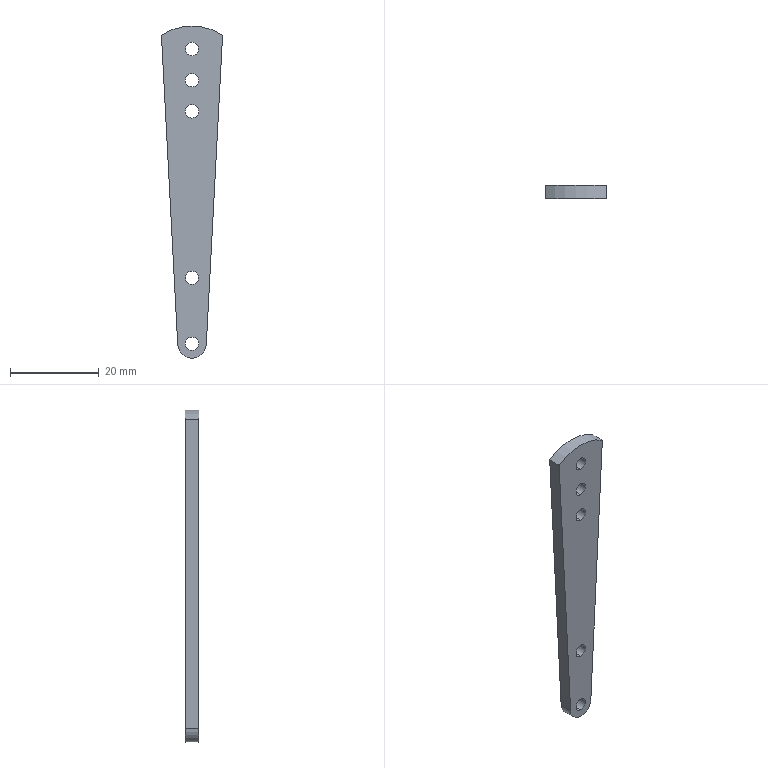Part | SolidWorks | features ICE 3, BaseBody 1 | 1 solid | 16 faces | box 13.735 x 3 x 74.656 mm | volume 2101 mm3 | cylinder 12 | plane 4 | commonest cylinder face diameters 3 x10 6.445 x1 24.375 x1
STEP:
#1=CARTESIAN_POINT('',(40.836,0.,-86.129));
#2=VERTEX_POINT('',#1);
#3=CARTESIAN_POINT('',(40.836,0.,-89.129));
#4=VERTEX_POINT('',#3);
#5=CARTESIAN_POINT('',(40.836,0.,-87.629));
#6=DIRECTION('',(0.,-1.,0.));
#7=DIRECTION('',(0.,0.,1.));
#8=AXIS2_PLACEMENT_3D('',#5,#6,#7);
#9=CIRCLE('',#8,1.5);
#10=EDGE_CURVE('',#2,#4,#9,.T.);
#11=ORIENTED_EDGE('',*,*,#10,.T.);
#12=CARTESIAN_POINT('',(40.836,3.,-89.129));
#13=VERTEX_POINT('',#12);
#14=CARTESIAN_POINT('',(40.836,-19.541,-89.129));
#15=DIRECTION('',(0.,1.,0.));
#16=VECTOR('',#15,1000.);
#17=LINE('',#14,#16);
#18=EDGE_CURVE('',#4,#13,#17,.T.);
#19=ORIENTED_EDGE('',*,*,#18,.T.);
#20=CARTESIAN_POINT('',(40.836,3.,-86.129));
#21=VERTEX_POINT('',#20);
#22=CARTESIAN_POINT('',(40.836,3.,-87.629));
#23=DIRECTION('',(0.,1.,0.));
#24=DIRECTION('',(0.,0.,1.));
#25=AXIS2_PLACEMENT_3D('',#22,#23,#24);
#26=CIRCLE('',#25,1.5);
#27=EDGE_CURVE('',#13,#21,#26,.T.);
#28=ORIENTED_EDGE('',*,*,#27,.T.);
#29=CARTESIAN_POINT('',(40.836,-19.541,-86.129));
#30=DIRECTION('',(0.,1.,0.));
#31=VECTOR('',#30,1000.);
#32=LINE('',#29,#31);
#33=EDGE_CURVE('',#2,#21,#32,.T.);
#34=ORIENTED_EDGE('',*,*,#33,.F.);
#35=EDGE_LOOP('',(#11,#19,#28,#34));
#36=FACE_OUTER_BOUND('',#35,.T.);
#37=CARTESIAN_POINT('',(40.836,-19.541,-87.629));
#38=DIRECTION('',(0.,1.,0.));
#39=DIRECTION('',(0.,0.,1.));
#40=AXIS2_PLACEMENT_3D('',#37,#38,#39);
#41=CYLINDRICAL_SURFACE('',#40,1.5);
#42=ADVANCED_FACE('',(#36),#41,.F.);
#43=CARTESIAN_POINT('',(40.836,0.,-71.309));
#44=VERTEX_POINT('',#43);
#45=CARTESIAN_POINT('',(40.836,0.,-74.309));
#46=VERTEX_POINT('',#45);
#47=CARTESIAN_POINT('',(40.836,0.,-72.809));
#48=DIRECTION('',(0.,-1.,0.));
#49=DIRECTION('',(0.,0.,1.));
#50=AXIS2_PLACEMENT_3D('',#47,#48,#49);
#51=CIRCLE('',#50,1.5);
#52=EDGE_CURVE('',#44,#46,#51,.T.);
#53=ORIENTED_EDGE('',*,*,#52,.T.);
#54=CARTESIAN_POINT('',(40.836,3.,-74.309));
#55=VERTEX_POINT('',#54);
#56=CARTESIAN_POINT('',(40.836,-39.423,-74.309));
#57=DIRECTION('',(0.,1.,0.));
#58=VECTOR('',#57,1000.);
#59=LINE('',#56,#58);
#60=EDGE_CURVE('',#46,#55,#59,.T.);
#61=ORIENTED_EDGE('',*,*,#60,.T.);
#62=CARTESIAN_POINT('',(40.836,3.,-71.309));
#63=VERTEX_POINT('',#62);
#64=CARTESIAN_POINT('',(40.836,3.,-72.809));
#65=DIRECTION('',(0.,1.,0.));
#66=DIRECTION('',(0.,0.,1.));
#67=AXIS2_PLACEMENT_3D('',#64,#65,#66);
#68=CIRCLE('',#67,1.5);
#69=EDGE_CURVE('',#55,#63,#68,.T.);
#70=ORIENTED_EDGE('',*,*,#69,.T.);
#71=CARTESIAN_POINT('',(40.836,-39.423,-71.309));
#72=DIRECTION('',(0.,1.,0.));
#73=VECTOR('',#72,1000.);
#74=LINE('',#71,#73);
#75=EDGE_CURVE('',#44,#63,#74,.T.);
#76=ORIENTED_EDGE('',*,*,#75,.F.);
#77=EDGE_LOOP('',(#53,#61,#70,#76));
#78=FACE_OUTER_BOUND('',#77,.T.);
#79=CARTESIAN_POINT('',(40.836,-39.423,-72.809));
#80=DIRECTION('',(0.,1.,0.));
#81=DIRECTION('',(0.,0.,1.));
#82=AXIS2_PLACEMENT_3D('',#79,#80,#81);
#83=CYLINDRICAL_SURFACE('',#82,1.5);
#84=ADVANCED_FACE('',(#78),#83,.F.);
#85=CARTESIAN_POINT('',(40.836,3.,-26.883));
#86=VERTEX_POINT('',#85);
#87=CARTESIAN_POINT('',(40.836,3.,-29.883));
#88=VERTEX_POINT('',#87);
#89=CARTESIAN_POINT('',(40.836,3.,-28.383));
#90=DIRECTION('',(0.,-1.,0.));
#91=DIRECTION('',(0.,0.,-1.));
#92=AXIS2_PLACEMENT_3D('',#89,#90,#91);
#93=CIRCLE('',#92,1.5);
#94=EDGE_CURVE('',#86,#88,#93,.T.);
#95=ORIENTED_EDGE('',*,*,#94,.F.);
#96=CARTESIAN_POINT('',(40.836,0.,-26.883));
#97=VERTEX_POINT('',#96);
#98=CARTESIAN_POINT('',(40.836,3.,-26.883));
#99=DIRECTION('',(0.,-1.,0.));
#100=VECTOR('',#99,1000.);
#101=LINE('',#98,#100);
#102=EDGE_CURVE('',#86,#97,#101,.T.);
#103=ORIENTED_EDGE('',*,*,#102,.T.);
#104=CARTESIAN_POINT('',(40.836,0.,-29.883));
#105=VERTEX_POINT('',#104);
#106=CARTESIAN_POINT('',(40.836,0.,-28.383));
#107=DIRECTION('',(0.,-1.,0.));
#108=DIRECTION('',(0.,0.,-1.));
#109=AXIS2_PLACEMENT_3D('',#106,#107,#108);
#110=CIRCLE('',#109,1.5);
#111=EDGE_CURVE('',#97,#105,#110,.T.);
#112=ORIENTED_EDGE('',*,*,#111,.T.);
#113=CARTESIAN_POINT('',(40.836,3.,-29.883));
#114=DIRECTION('',(0.,-1.,0.));
#115=VECTOR('',#114,1000.);
#116=LINE('',#113,#115);
#117=EDGE_CURVE('',#88,#105,#116,.T.);
#118=ORIENTED_EDGE('',*,*,#117,.F.);
#119=EDGE_LOOP('',(#95,#103,#112,#118));
#120=FACE_OUTER_BOUND('',#119,.T.);
#121=CARTESIAN_POINT('',(40.836,3.,-28.383));
#122=DIRECTION('',(0.,-1.,0.));
#123=DIRECTION('',(0.,0.,-1.));
#124=AXIS2_PLACEMENT_3D('',#121,#122,#123);
#125=CYLINDRICAL_SURFACE('',#124,1.5);
#126=ADVANCED_FACE('',(#120),#125,.F.);
#127=CARTESIAN_POINT('',(40.836,3.,-19.883));
#128=VERTEX_POINT('',#127);
#129=CARTESIAN_POINT('',(40.836,3.,-22.883));
#130=VERTEX_POINT('',#129);
#131=CARTESIAN_POINT('',(40.836,3.,-21.383));
#132=DIRECTION('',(0.,-1.,0.));
#133=DIRECTION('',(0.,0.,-1.));
#134=AXIS2_PLACEMENT_3D('',#131,#132,#133);
#135=CIRCLE('',#134,1.5);
#136=EDGE_CURVE('',#128,#130,#135,.T.);
#137=ORIENTED_EDGE('',*,*,#136,.F.);
#138=CARTESIAN_POINT('',(40.836,0.,-19.883));
#139=VERTEX_POINT('',#138);
#140=CARTESIAN_POINT('',(40.836,3.,-19.883));
#141=DIRECTION('',(0.,-1.,0.));
#142=VECTOR('',#141,1000.);
#143=LINE('',#140,#142);
#144=EDGE_CURVE('',#128,#139,#143,.T.);
#145=ORIENTED_EDGE('',*,*,#144,.T.);
#146=CARTESIAN_POINT('',(40.836,0.,-22.883));
#147=VERTEX_POINT('',#146);
#148=CARTESIAN_POINT('',(40.836,0.,-21.383));
#149=DIRECTION('',(0.,-1.,0.));
#150=DIRECTION('',(0.,0.,-1.));
#151=AXIS2_PLACEMENT_3D('',#148,#149,#150);
#152=CIRCLE('',#151,1.5);
#153=EDGE_CURVE('',#139,#147,#152,.T.);
#154=ORIENTED_EDGE('',*,*,#153,.T.);
#155=CARTESIAN_POINT('',(40.836,3.,-22.883));
#156=DIRECTION('',(0.,-1.,0.));
#157=VECTOR('',#156,1000.);
#158=LINE('',#155,#157);
#159=EDGE_CURVE('',#130,#147,#158,.T.);
#160=ORIENTED_EDGE('',*,*,#159,.F.);
#161=EDGE_LOOP('',(#137,#145,#154,#160));
#162=FACE_OUTER_BOUND('',#161,.T.);
#163=CARTESIAN_POINT('',(40.836,3.,-21.383));
#164=DIRECTION('',(0.,-1.,0.));
#165=DIRECTION('',(0.,0.,-1.));
#166=AXIS2_PLACEMENT_3D('',#163,#164,#165);
#167=CYLINDRICAL_SURFACE('',#166,1.5);
#168=ADVANCED_FACE('',(#162),#167,.F.);
#169=CARTESIAN_POINT('',(40.836,3.,-33.883));
#170=VERTEX_POINT('',#169);
#171=CARTESIAN_POINT('',(40.836,3.,-36.883));
#172=VERTEX_POINT('',#171);
#173=CARTESIAN_POINT('',(40.836,3.,-35.383));
#174=DIRECTION('',(0.,-1.,0.));
#175=DIRECTION('',(0.,0.,-1.));
#176=AXIS2_PLACEMENT_3D('',#173,#174,#175);
#177=CIRCLE('',#176,1.5);
#178=EDGE_CURVE('',#170,#172,#177,.T.);
#179=ORIENTED_EDGE('',*,*,#178,.F.);
#180=CARTESIAN_POINT('',(40.836,0.,-33.883));
#181=VERTEX_POINT('',#180);
#182=CARTESIAN_POINT('',(40.836,3.,-33.883));
#183=DIRECTION('',(0.,-1.,0.));
#184=VECTOR('',#183,1000.);
#185=LINE('',#182,#184);
#186=EDGE_CURVE('',#170,#181,#185,.T.);
#187=ORIENTED_EDGE('',*,*,#186,.T.);
#188=CARTESIAN_POINT('',(40.836,0.,-36.883));
#189=VERTEX_POINT('',#188);
#190=CARTESIAN_POINT('',(40.836,0.,-35.383));
#191=DIRECTION('',(0.,-1.,0.));
#192=DIRECTION('',(0.,0.,-1.));
#193=AXIS2_PLACEMENT_3D('',#190,#191,#192);
#194=CIRCLE('',#193,1.5);
#195=EDGE_CURVE('',#181,#189,#194,.T.);
#196=ORIENTED_EDGE('',*,*,#195,.T.);
#197=CARTESIAN_POINT('',(40.836,3.,-36.883));
#198=DIRECTION('',(0.,-1.,0.));
#199=VECTOR('',#198,1000.);
#200=LINE('',#197,#199);
#201=EDGE_CURVE('',#172,#189,#200,.T.);
#202=ORIENTED_EDGE('',*,*,#201,.F.);
#203=EDGE_LOOP('',(#179,#187,#196,#202));
#204=FACE_OUTER_BOUND('',#203,.T.);
#205=CARTESIAN_POINT('',(40.836,3.,-35.383));
#206=DIRECTION('',(0.,-1.,0.));
#207=DIRECTION('',(0.,0.,-1.));
#208=AXIS2_PLACEMENT_3D('',#205,#206,#207);
#209=CYLINDRICAL_SURFACE('',#208,1.5);
#210=ADVANCED_FACE('',(#204),#209,.F.);
#211=CARTESIAN_POINT('',(44.054,3.,-87.798));
#212=VERTEX_POINT('',#211);
#213=CARTESIAN_POINT('',(47.703,3.,-18.315));
#214=VERTEX_POINT('',#213);
#215=CARTESIAN_POINT('',(45.586,3.,-58.633));
#216=DIRECTION('',(0.05245,0.,0.9986));
#217=VECTOR('',#216,1000.);
#218=LINE('',#215,#217);
#219=EDGE_CURVE('',#212,#214,#218,.T.);
#220=ORIENTED_EDGE('',*,*,#219,.F.);
#221=CARTESIAN_POINT('',(37.617,3.,-87.798));
#222=VERTEX_POINT('',#221);
#223=CARTESIAN_POINT('',(40.836,3.,-87.629));
#224=DIRECTION('',(0.,1.,0.));
#225=DIRECTION('',(0.,0.,-1.));
#226=AXIS2_PLACEMENT_3D('',#223,#224,#225);
#227=CIRCLE('',#226,3.223);
#228=EDGE_CURVE('',#212,#222,#227,.T.);
#229=ORIENTED_EDGE('',*,*,#228,.T.);
#230=CARTESIAN_POINT('',(33.968,3.,-18.315));
#231=VERTEX_POINT('',#230);
#232=CARTESIAN_POINT('',(36.086,3.,-58.633));
#233=DIRECTION('',(0.05245,0.,-0.9986));
#234=VECTOR('',#233,1000.);
#235=LINE('',#232,#234);
#236=EDGE_CURVE('',#231,#222,#235,.T.);
#237=ORIENTED_EDGE('',*,*,#236,.F.);
#238=CARTESIAN_POINT('',(40.836,3.,-28.383));
#239=DIRECTION('',(0.,-1.,0.));
#240=DIRECTION('',(0.,0.,-1.));
#241=AXIS2_PLACEMENT_3D('',#238,#239,#240);
#242=CIRCLE('',#241,12.188);
#243=EDGE_CURVE('',#214,#231,#242,.T.);
#244=ORIENTED_EDGE('',*,*,#243,.F.);
#245=EDGE_LOOP('',(#220,#229,#237,#244));
#246=FACE_OUTER_BOUND('',#245,.T.);
#247=CARTESIAN_POINT('',(40.836,3.,-35.383));
#248=DIRECTION('',(0.,-1.,0.));
#249=DIRECTION('',(0.,0.,-1.));
#250=AXIS2_PLACEMENT_3D('',#247,#248,#249);
#251=CIRCLE('',#250,1.5);
#252=EDGE_CURVE('',#172,#170,#251,.T.);
#253=ORIENTED_EDGE('',*,*,#252,.T.);
#254=ORIENTED_EDGE('',*,*,#178,.T.);
#255=EDGE_LOOP('',(#253,#254));
#256=FACE_BOUND('',#255,.T.);
#257=CARTESIAN_POINT('',(40.836,3.,-21.383));
#258=DIRECTION('',(0.,-1.,0.));
#259=DIRECTION('',(0.,0.,-1.));
#260=AXIS2_PLACEMENT_3D('',#257,#258,#259);
#261=CIRCLE('',#260,1.5);
#262=EDGE_CURVE('',#130,#128,#261,.T.);
#263=ORIENTED_EDGE('',*,*,#262,.T.);
#264=ORIENTED_EDGE('',*,*,#136,.T.);
#265=EDGE_LOOP('',(#263,#264));
#266=FACE_BOUND('',#265,.T.);
#267=CARTESIAN_POINT('',(40.836,3.,-28.383));
#268=DIRECTION('',(0.,-1.,0.));
#269=DIRECTION('',(0.,0.,-1.));
#270=AXIS2_PLACEMENT_3D('',#267,#268,#269);
#271=CIRCLE('',#270,1.5);
#272=EDGE_CURVE('',#88,#86,#271,.T.);
#273=ORIENTED_EDGE('',*,*,#272,.T.);
#274=ORIENTED_EDGE('',*,*,#94,.T.);
#275=EDGE_LOOP('',(#273,#274));
#276=FACE_BOUND('',#275,.T.);
#277=CARTESIAN_POINT('',(40.836,3.,-72.809));
#278=DIRECTION('',(0.,1.,0.));
#279=DIRECTION('',(0.,0.,1.));
#280=AXIS2_PLACEMENT_3D('',#277,#278,#279);
#281=CIRCLE('',#280,1.5);
#282=EDGE_CURVE('',#63,#55,#281,.T.);
#283=ORIENTED_EDGE('',*,*,#282,.F.);
#284=ORIENTED_EDGE('',*,*,#69,.F.);
#285=EDGE_LOOP('',(#283,#284));
#286=FACE_BOUND('',#285,.T.);
#287=CARTESIAN_POINT('',(40.836,3.,-87.629));
#288=DIRECTION('',(0.,1.,0.));
#289=DIRECTION('',(0.,0.,1.));
#290=AXIS2_PLACEMENT_3D('',#287,#288,#289);
#291=CIRCLE('',#290,1.5);
#292=EDGE_CURVE('',#21,#13,#291,.T.);
#293=ORIENTED_EDGE('',*,*,#292,.F.);
#294=ORIENTED_EDGE('',*,*,#27,.F.);
#295=EDGE_LOOP('',(#293,#294));
#296=FACE_BOUND('',#295,.T.);
#297=CARTESIAN_POINT('',(42.689,3.,-41.89));
#298=DIRECTION('',(0.,1.,0.));
#299=DIRECTION('',(1.,0.,0.));
#300=AXIS2_PLACEMENT_3D('',#297,#298,#299);
#301=PLANE('',#300);
#302=ADVANCED_FACE('',(#246,#256,#266,#276,#286,#296),#301,.T.);
#303=CARTESIAN_POINT('',(37.617,0.,-87.798));
#304=VERTEX_POINT('',#303);
#305=CARTESIAN_POINT('',(44.054,0.,-87.798));
#306=VERTEX_POINT('',#305);
#307=CARTESIAN_POINT('',(40.836,0.,-87.629));
#308=DIRECTION('',(0.,-1.,0.));
#309=DIRECTION('',(0.,0.,1.));
#310=AXIS2_PLACEMENT_3D('',#307,#308,#309);
#311=CIRCLE('',#310,3.223);
#312=EDGE_CURVE('',#304,#306,#311,.T.);
#313=ORIENTED_EDGE('',*,*,#312,.T.);
#314=CARTESIAN_POINT('',(47.703,0.,-18.315));
#315=VERTEX_POINT('',#314);
#316=CARTESIAN_POINT('',(45.586,0.,-58.633));
#317=DIRECTION('',(0.05245,0.,0.9986));
#318=VECTOR('',#317,1000.);
#319=LINE('',#316,#318);
#320=EDGE_CURVE('',#306,#315,#319,.T.);
#321=ORIENTED_EDGE('',*,*,#320,.T.);
#322=CARTESIAN_POINT('',(33.968,0.,-18.315));
#323=VERTEX_POINT('',#322);
#324=CARTESIAN_POINT('',(40.836,0.,-28.383));
#325=DIRECTION('',(0.,-1.,0.));
#326=DIRECTION('',(0.,0.,-1.));
#327=AXIS2_PLACEMENT_3D('',#324,#325,#326);
#328=CIRCLE('',#327,12.188);
#329=EDGE_CURVE('',#315,#323,#328,.T.);
#330=ORIENTED_EDGE('',*,*,#329,.T.);
#331=CARTESIAN_POINT('',(36.086,0.,-58.633));
#332=DIRECTION('',(0.05245,0.,-0.9986));
#333=VECTOR('',#332,1000.);
#334=LINE('',#331,#333);
#335=EDGE_CURVE('',#323,#304,#334,.T.);
#336=ORIENTED_EDGE('',*,*,#335,.T.);
#337=EDGE_LOOP('',(#313,#321,#330,#336));
#338=FACE_OUTER_BOUND('',#337,.T.);
#339=CARTESIAN_POINT('',(40.836,0.,-35.383));
#340=DIRECTION('',(0.,-1.,0.));
#341=DIRECTION('',(0.,0.,-1.));
#342=AXIS2_PLACEMENT_3D('',#339,#340,#341);
#343=CIRCLE('',#342,1.5);
#344=EDGE_CURVE('',#189,#181,#343,.T.);
#345=ORIENTED_EDGE('',*,*,#344,.F.);
#346=ORIENTED_EDGE('',*,*,#195,.F.);
#347=EDGE_LOOP('',(#345,#346));
#348=FACE_BOUND('',#347,.T.);
#349=CARTESIAN_POINT('',(40.836,0.,-21.383));
#350=DIRECTION('',(0.,-1.,0.));
#351=DIRECTION('',(0.,0.,-1.));
#352=AXIS2_PLACEMENT_3D('',#349,#350,#351);
#353=CIRCLE('',#352,1.5);
#354=EDGE_CURVE('',#147,#139,#353,.T.);
#355=ORIENTED_EDGE('',*,*,#354,.F.);
#356=ORIENTED_EDGE('',*,*,#153,.F.);
#357=EDGE_LOOP('',(#355,#356));
#358=FACE_BOUND('',#357,.T.);
#359=CARTESIAN_POINT('',(40.836,0.,-28.383));
#360=DIRECTION('',(0.,-1.,0.));
#361=DIRECTION('',(0.,0.,-1.));
#362=AXIS2_PLACEMENT_3D('',#359,#360,#361);
#363=CIRCLE('',#362,1.5);
#364=EDGE_CURVE('',#105,#97,#363,.T.);
#365=ORIENTED_EDGE('',*,*,#364,.F.);
#366=ORIENTED_EDGE('',*,*,#111,.F.);
#367=EDGE_LOOP('',(#365,#366));
#368=FACE_BOUND('',#367,.T.);
#369=ORIENTED_EDGE('',*,*,#52,.F.);
#370=CARTESIAN_POINT('',(40.836,0.,-72.809));
#371=DIRECTION('',(0.,-1.,0.));
#372=DIRECTION('',(0.,0.,1.));
#373=AXIS2_PLACEMENT_3D('',#370,#371,#372);
#374=CIRCLE('',#373,1.5);
#375=EDGE_CURVE('',#46,#44,#374,.T.);
#376=ORIENTED_EDGE('',*,*,#375,.F.);
#377=EDGE_LOOP('',(#369,#376));
#378=FACE_BOUND('',#377,.T.);
#379=ORIENTED_EDGE('',*,*,#10,.F.);
#380=CARTESIAN_POINT('',(40.836,0.,-87.629));
#381=DIRECTION('',(0.,-1.,0.));
#382=DIRECTION('',(0.,0.,1.));
#383=AXIS2_PLACEMENT_3D('',#380,#381,#382);
#384=CIRCLE('',#383,1.5);
#385=EDGE_CURVE('',#4,#2,#384,.T.);
#386=ORIENTED_EDGE('',*,*,#385,.F.);
#387=EDGE_LOOP('',(#379,#386));
#388=FACE_BOUND('',#387,.T.);
#389=CARTESIAN_POINT('',(42.689,0.,-41.89));
#390=DIRECTION('',(0.,1.,0.));
#391=DIRECTION('',(1.,0.,0.));
#392=AXIS2_PLACEMENT_3D('',#389,#390,#391);
#393=PLANE('',#392);
#394=ADVANCED_FACE('',(#338,#348,#358,#368,#378,#388),#393,.F.);
#395=ORIENTED_EDGE('',*,*,#186,.F.);
#396=ORIENTED_EDGE('',*,*,#252,.F.);
#397=ORIENTED_EDGE('',*,*,#201,.T.);
#398=ORIENTED_EDGE('',*,*,#344,.T.);
#399=EDGE_LOOP('',(#395,#396,#397,#398));
#400=FACE_OUTER_BOUND('',#399,.T.);
#401=CARTESIAN_POINT('',(40.836,3.,-35.383));
#402=DIRECTION('',(0.,-1.,0.));
#403=DIRECTION('',(0.,0.,-1.));
#404=AXIS2_PLACEMENT_3D('',#401,#402,#403);
#405=CYLINDRICAL_SURFACE('',#404,1.5);
#406=ADVANCED_FACE('',(#400),#405,.F.);
#407=ORIENTED_EDGE('',*,*,#144,.F.);
#408=ORIENTED_EDGE('',*,*,#262,.F.);
#409=ORIENTED_EDGE('',*,*,#159,.T.);
#410=ORIENTED_EDGE('',*,*,#354,.T.);
#411=EDGE_LOOP('',(#407,#408,#409,#410));
#412=FACE_OUTER_BOUND('',#411,.T.);
#413=CARTESIAN_POINT('',(40.836,3.,-21.383));
#414=DIRECTION('',(0.,-1.,0.));
#415=DIRECTION('',(0.,0.,-1.));
#416=AXIS2_PLACEMENT_3D('',#413,#414,#415);
#417=CYLINDRICAL_SURFACE('',#416,1.5);
#418=ADVANCED_FACE('',(#412),#417,.F.);
#419=ORIENTED_EDGE('',*,*,#102,.F.);
#420=ORIENTED_EDGE('',*,*,#272,.F.);
#421=ORIENTED_EDGE('',*,*,#117,.T.);
#422=ORIENTED_EDGE('',*,*,#364,.T.);
#423=EDGE_LOOP('',(#419,#420,#421,#422));
#424=FACE_OUTER_BOUND('',#423,.T.);
#425=CARTESIAN_POINT('',(40.836,3.,-28.383));
#426=DIRECTION('',(0.,-1.,0.));
#427=DIRECTION('',(0.,0.,-1.));
#428=AXIS2_PLACEMENT_3D('',#425,#426,#427);
#429=CYLINDRICAL_SURFACE('',#428,1.5);
#430=ADVANCED_FACE('',(#424),#429,.F.);
#431=CARTESIAN_POINT('',(47.703,-7.,-18.315));
#432=DIRECTION('',(0.,1.,0.));
#433=VECTOR('',#432,1000.);
#434=LINE('',#431,#433);
#435=EDGE_CURVE('',#315,#214,#434,.T.);
#436=ORIENTED_EDGE('',*,*,#435,.T.);
#437=ORIENTED_EDGE('',*,*,#243,.T.);
#438=CARTESIAN_POINT('',(33.968,-7.,-18.315));
#439=DIRECTION('',(0.,1.,0.));
#440=VECTOR('',#439,1000.);
#441=LINE('',#438,#440);
#442=EDGE_CURVE('',#323,#231,#441,.T.);
#443=ORIENTED_EDGE('',*,*,#442,.F.);
#444=ORIENTED_EDGE('',*,*,#329,.F.);
#445=EDGE_LOOP('',(#436,#437,#443,#444));
#446=FACE_OUTER_BOUND('',#445,.T.);
#447=CARTESIAN_POINT('',(40.836,3.,-28.383));
#448=DIRECTION('',(0.,-1.,0.));
#449=DIRECTION('',(0.,0.,-1.));
#450=AXIS2_PLACEMENT_3D('',#447,#448,#449);
#451=CYLINDRICAL_SURFACE('',#450,12.188);
#452=ADVANCED_FACE('',(#446),#451,.T.);
#453=ORIENTED_EDGE('',*,*,#335,.F.);
#454=ORIENTED_EDGE('',*,*,#442,.T.);
#455=ORIENTED_EDGE('',*,*,#236,.T.);
#456=CARTESIAN_POINT('',(37.617,-19.541,-87.798));
#457=DIRECTION('',(0.,1.,0.));
#458=VECTOR('',#457,1000.);
#459=LINE('',#456,#458);
#460=EDGE_CURVE('',#304,#222,#459,.T.);
#461=ORIENTED_EDGE('',*,*,#460,.F.);
#462=EDGE_LOOP('',(#453,#454,#455,#461));
#463=FACE_OUTER_BOUND('',#462,.T.);
#464=CARTESIAN_POINT('',(36.086,3.,-58.633));
#465=DIRECTION('',(-0.9986,0.,-0.05245));
#466=DIRECTION('',(-0.05245,0.,0.9986));
#467=AXIS2_PLACEMENT_3D('',#464,#465,#466);
#468=PLANE('',#467);
#469=ADVANCED_FACE('',(#463),#468,.T.);
#470=ORIENTED_EDGE('',*,*,#219,.T.);
#471=ORIENTED_EDGE('',*,*,#435,.F.);
#472=ORIENTED_EDGE('',*,*,#320,.F.);
#473=CARTESIAN_POINT('',(44.054,-19.541,-87.798));
#474=DIRECTION('',(0.,1.,0.));
#475=VECTOR('',#474,1000.);
#476=LINE('',#473,#475);
#477=EDGE_CURVE('',#306,#212,#476,.T.);
#478=ORIENTED_EDGE('',*,*,#477,.T.);
#479=EDGE_LOOP('',(#470,#471,#472,#478));
#480=FACE_OUTER_BOUND('',#479,.T.);
#481=CARTESIAN_POINT('',(45.586,3.,-58.633));
#482=DIRECTION('',(0.9986,0.,-0.05245));
#483=DIRECTION('',(0.,-1.,0.));
#484=AXIS2_PLACEMENT_3D('',#481,#482,#483);
#485=PLANE('',#484);
#486=ADVANCED_FACE('',(#480),#485,.T.);
#487=ORIENTED_EDGE('',*,*,#60,.F.);
#488=ORIENTED_EDGE('',*,*,#375,.T.);
#489=ORIENTED_EDGE('',*,*,#75,.T.);
#490=ORIENTED_EDGE('',*,*,#282,.T.);
#491=EDGE_LOOP('',(#487,#488,#489,#490));
#492=FACE_OUTER_BOUND('',#491,.T.);
#493=CARTESIAN_POINT('',(40.836,-39.423,-72.809));
#494=DIRECTION('',(0.,1.,0.));
#495=DIRECTION('',(0.,0.,1.));
#496=AXIS2_PLACEMENT_3D('',#493,#494,#495);
#497=CYLINDRICAL_SURFACE('',#496,1.5);
#498=ADVANCED_FACE('',(#492),#497,.F.);
#499=ORIENTED_EDGE('',*,*,#312,.F.);
#500=ORIENTED_EDGE('',*,*,#460,.T.);
#501=ORIENTED_EDGE('',*,*,#228,.F.);
#502=ORIENTED_EDGE('',*,*,#477,.F.);
#503=EDGE_LOOP('',(#499,#500,#501,#502));
#504=FACE_OUTER_BOUND('',#503,.T.);
#505=CARTESIAN_POINT('',(40.836,-19.541,-87.629));
#506=DIRECTION('',(0.,1.,0.));
#507=DIRECTION('',(0.,0.,1.));
#508=AXIS2_PLACEMENT_3D('',#505,#506,#507);
#509=CYLINDRICAL_SURFACE('',#508,3.223);
#510=ADVANCED_FACE('',(#504),#509,.T.);
#511=ORIENTED_EDGE('',*,*,#18,.F.);
#512=ORIENTED_EDGE('',*,*,#385,.T.);
#513=ORIENTED_EDGE('',*,*,#33,.T.);
#514=ORIENTED_EDGE('',*,*,#292,.T.);
#515=EDGE_LOOP('',(#511,#512,#513,#514));
#516=FACE_OUTER_BOUND('',#515,.T.);
#517=CARTESIAN_POINT('',(40.836,-19.541,-87.629));
#518=DIRECTION('',(0.,1.,0.));
#519=DIRECTION('',(0.,0.,1.));
#520=AXIS2_PLACEMENT_3D('',#517,#518,#519);
#521=CYLINDRICAL_SURFACE('',#520,1.5);
#522=ADVANCED_FACE('',(#516),#521,.F.);
#523=CLOSED_SHELL('',(#42,#84,#126,#168,#210,#302,#394,#406,#418,#430,#452,#469,#486,#498,#510,#522));
#524=MANIFOLD_SOLID_BREP('',#523);
#525=CARTESIAN_POINT('',(0.,0.,0.));
#526=DIRECTION('',(0.,0.,1.));
#527=DIRECTION('',(1.,0.,0.));
#528=AXIS2_PLACEMENT_3D('',#525,#526,#527);
#529=(LENGTH_UNIT()NAMED_UNIT(*)SI_UNIT(.MILLI.,.METRE.));
#530=UNCERTAINTY_MEASURE_WITH_UNIT(LENGTH_MEASURE(0.00001),#529,'','');
#531=(NAMED_UNIT(*)PLANE_ANGLE_UNIT()SI_UNIT($,.RADIAN.));
#532=(NAMED_UNIT(*)SI_UNIT($,.STERADIAN.)SOLID_ANGLE_UNIT());
#533=(GEOMETRIC_REPRESENTATION_CONTEXT(3)GLOBAL_UNCERTAINTY_ASSIGNED_CONTEXT((#530))GLOBAL_UNIT_ASSIGNED_CONTEXT((#529,#531,#532))REPRESENTATION_CONTEXT('',''));
#534=ADVANCED_BREP_SHAPE_REPRESENTATION('',(#524,#528),#533);